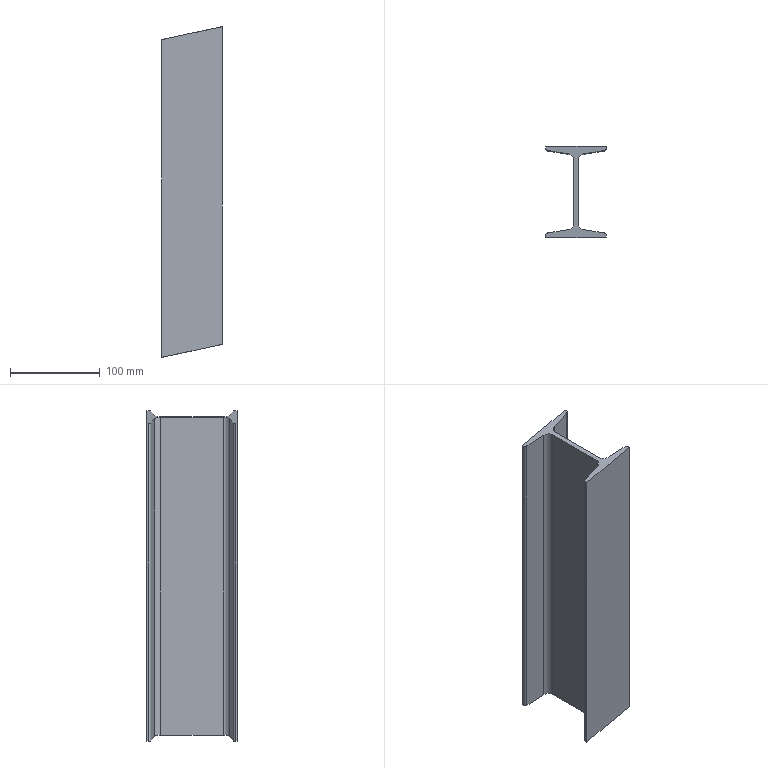Part | SolidWorks | features BaseBody 1 | 1 solid | 22 faces | box 67.6 x 101.6 x 369.5 mm | volume 493243 mm3 | plane 14 | cylinder 8 | commonest cylinder face diameters 5.6 x4 14.8 x4
STEP:
#1=CARTESIAN_POINT('',(50.959,42.223,361.667));
#2=VERTEX_POINT('',#1);
#3=CARTESIAN_POINT('',(50.959,112.103,361.667));
#4=VERTEX_POINT('',#3);
#5=CARTESIAN_POINT('',(50.959,42.223,361.667));
#6=DIRECTION('',(0.,1.,0.));
#7=VECTOR('',#6,1000.);
#8=LINE('',#5,#7);
#9=EDGE_CURVE('',#2,#4,#8,.T.);
#10=ORIENTED_EDGE('',*,*,#9,.T.);
#11=CARTESIAN_POINT('',(50.959,112.103,6.795));
#12=VERTEX_POINT('',#11);
#13=CARTESIAN_POINT('',(50.959,112.103,0.));
#14=DIRECTION('',(0.,0.,-1.));
#15=VECTOR('',#14,1000.);
#16=LINE('',#13,#15);
#17=EDGE_CURVE('',#4,#12,#16,.T.);
#18=ORIENTED_EDGE('',*,*,#17,.T.);
#19=CARTESIAN_POINT('',(50.959,42.223,6.795));
#20=VERTEX_POINT('',#19);
#21=CARTESIAN_POINT('',(50.959,42.223,6.795));
#22=DIRECTION('',(0.,-1.,0.));
#23=VECTOR('',#22,1000.);
#24=LINE('',#21,#23);
#25=EDGE_CURVE('',#12,#20,#24,.T.);
#26=ORIENTED_EDGE('',*,*,#25,.T.);
#27=CARTESIAN_POINT('',(50.959,42.223,0.));
#28=DIRECTION('',(0.,0.,1.));
#29=VECTOR('',#28,1000.);
#30=LINE('',#27,#29);
#31=EDGE_CURVE('',#20,#2,#30,.T.);
#32=ORIENTED_EDGE('',*,*,#31,.T.);
#33=EDGE_LOOP('',(#10,#18,#26,#32));
#34=FACE_OUTER_BOUND('',#33,.T.);
#35=CARTESIAN_POINT('',(50.959,42.223,0.));
#36=DIRECTION('',(-1.,0.,0.));
#37=DIRECTION('',(0.,0.,1.));
#38=AXIS2_PLACEMENT_3D('',#35,#36,#37);
#39=PLANE('',#38);
#40=ADVANCED_FACE('',(#34),#39,.T.);
#41=ORIENTED_EDGE('',*,*,#17,.F.);
#42=CARTESIAN_POINT('',(44.781,119.402,360.33));
#43=VERTEX_POINT('',#42);
#44=CARTESIAN_POINT('',(44.781,119.402,360.33));
#45=CARTESIAN_POINT('',(48.514,118.777,361.137));
#46=CARTESIAN_POINT('',(50.959,115.888,361.667));
#47=CARTESIAN_POINT('',(50.959,112.103,361.667));
#48=(BOUNDED_CURVE()B_SPLINE_CURVE(3,(#44,#45,#46,#47),.UNSPECIFIED.,.F.,.T.)B_SPLINE_CURVE_WITH_KNOTS((4,4),(4.878,6.283),.UNSPECIFIED.)CURVE()GEOMETRIC_REPRESENTATION_ITEM()RATIONAL_B_SPLINE_CURVE((1.,0.8422,0.8422,1.))REPRESENTATION_ITEM(''));
#49=EDGE_CURVE('',#43,#4,#48,.T.);
#50=ORIENTED_EDGE('',*,*,#49,.F.);
#51=CARTESIAN_POINT('',(44.781,119.402,5.458));
#52=VERTEX_POINT('',#51);
#53=CARTESIAN_POINT('',(44.781,119.402,0.));
#54=DIRECTION('',(0.,0.,1.));
#55=VECTOR('',#54,1000.);
#56=LINE('',#53,#55);
#57=EDGE_CURVE('',#52,#43,#56,.T.);
#58=ORIENTED_EDGE('',*,*,#57,.F.);
#59=CARTESIAN_POINT('',(50.959,112.103,6.795));
#60=CARTESIAN_POINT('',(50.959,115.888,6.795));
#61=CARTESIAN_POINT('',(48.514,118.777,6.265));
#62=CARTESIAN_POINT('',(44.781,119.402,5.458));
#63=(BOUNDED_CURVE()B_SPLINE_CURVE(3,(#59,#60,#61,#62),.UNSPECIFIED.,.F.,.T.)B_SPLINE_CURVE_WITH_KNOTS((4,4),(0.,1.405),.UNSPECIFIED.)CURVE()GEOMETRIC_REPRESENTATION_ITEM()RATIONAL_B_SPLINE_CURVE((1.,0.8422,0.8422,1.))REPRESENTATION_ITEM(''));
#64=EDGE_CURVE('',#12,#52,#63,.T.);
#65=ORIENTED_EDGE('',*,*,#64,.F.);
#66=EDGE_LOOP('',(#41,#50,#58,#65));
#67=FACE_OUTER_BOUND('',#66,.T.);
#68=CARTESIAN_POINT('',(43.559,112.103,0.));
#69=DIRECTION('',(0.,0.,1.));
#70=DIRECTION('',(1.,0.,0.));
#71=AXIS2_PLACEMENT_3D('',#68,#69,#70);
#72=CYLINDRICAL_SURFACE('',#71,7.4);
#73=ADVANCED_FACE('',(#67),#72,.F.);
#74=CARTESIAN_POINT('',(87.159,26.363,369.5));
#75=VERTEX_POINT('',#74);
#76=CARTESIAN_POINT('',(19.559,26.363,354.872));
#77=VERTEX_POINT('',#76);
#78=CARTESIAN_POINT('',(4.183,26.363,351.545));
#79=DIRECTION('',(-0.9774,0.,-0.2115));
#80=VECTOR('',#79,1000.);
#81=LINE('',#78,#80);
#82=EDGE_CURVE('',#75,#77,#81,.T.);
#83=ORIENTED_EDGE('',*,*,#82,.F.);
#84=CARTESIAN_POINT('',(87.159,28.334,369.5));
#85=VERTEX_POINT('',#84);
#86=CARTESIAN_POINT('',(87.159,26.363,369.5));
#87=DIRECTION('',(0.,-1.,0.));
#88=VECTOR('',#87,1000.);
#89=LINE('',#86,#88);
#90=EDGE_CURVE('',#85,#75,#89,.T.);
#91=ORIENTED_EDGE('',*,*,#90,.F.);
#92=CARTESIAN_POINT('',(84.821,31.095,368.994));
#93=VERTEX_POINT('',#92);
#94=CARTESIAN_POINT('',(84.821,31.095,368.994));
#95=CARTESIAN_POINT('',(86.234,30.859,369.3));
#96=CARTESIAN_POINT('',(87.159,29.766,369.5));
#97=CARTESIAN_POINT('',(87.159,28.334,369.5));
#98=(BOUNDED_CURVE()B_SPLINE_CURVE(3,(#94,#95,#96,#97),.UNSPECIFIED.,.F.,.T.)B_SPLINE_CURVE_WITH_KNOTS((4,4),(4.878,6.283),.UNSPECIFIED.)CURVE()GEOMETRIC_REPRESENTATION_ITEM()RATIONAL_B_SPLINE_CURVE((1.,0.8422,0.8422,1.))REPRESENTATION_ITEM(''));
#99=EDGE_CURVE('',#93,#85,#98,.T.);
#100=ORIENTED_EDGE('',*,*,#99,.F.);
#101=CARTESIAN_POINT('',(61.938,34.925,364.042));
#102=VERTEX_POINT('',#101);
#103=CARTESIAN_POINT('',(61.938,34.925,364.042));
#104=DIRECTION('',(0.9646,-0.1614,0.2087));
#105=VECTOR('',#104,1000.);
#106=LINE('',#103,#105);
#107=EDGE_CURVE('',#102,#93,#106,.T.);
#108=ORIENTED_EDGE('',*,*,#107,.F.);
#109=CARTESIAN_POINT('',(55.759,42.223,362.705));
#110=VERTEX_POINT('',#109);
#111=CARTESIAN_POINT('',(55.759,42.223,362.705));
#112=CARTESIAN_POINT('',(55.759,38.438,362.705));
#113=CARTESIAN_POINT('',(58.205,35.55,363.235));
#114=CARTESIAN_POINT('',(61.938,34.925,364.042));
#115=(BOUNDED_CURVE()B_SPLINE_CURVE(3,(#111,#112,#113,#114),.UNSPECIFIED.,.F.,.F.)B_SPLINE_CURVE_WITH_KNOTS((4,4),(3.142,4.547),.UNSPECIFIED.)CURVE()GEOMETRIC_REPRESENTATION_ITEM()RATIONAL_B_SPLINE_CURVE((1.,0.8422,0.8422,1.))REPRESENTATION_ITEM(''));
#116=EDGE_CURVE('',#110,#102,#115,.T.);
#117=ORIENTED_EDGE('',*,*,#116,.F.);
#118=CARTESIAN_POINT('',(55.759,112.103,362.705));
#119=VERTEX_POINT('',#118);
#120=CARTESIAN_POINT('',(55.759,26.363,362.705));
#121=DIRECTION('',(0.,-1.,0.));
#122=VECTOR('',#121,1000.);
#123=LINE('',#120,#122);
#124=EDGE_CURVE('',#119,#110,#123,.T.);
#125=ORIENTED_EDGE('',*,*,#124,.F.);
#126=CARTESIAN_POINT('',(61.938,119.402,364.042));
#127=VERTEX_POINT('',#126);
#128=CARTESIAN_POINT('',(61.938,119.402,364.042));
#129=CARTESIAN_POINT('',(58.205,118.777,363.235));
#130=CARTESIAN_POINT('',(55.759,115.888,362.705));
#131=CARTESIAN_POINT('',(55.759,112.103,362.705));
#132=(BOUNDED_CURVE()B_SPLINE_CURVE(3,(#128,#129,#130,#131),.UNSPECIFIED.,.F.,.T.)B_SPLINE_CURVE_WITH_KNOTS((4,4),(1.737,3.142),.UNSPECIFIED.)CURVE()GEOMETRIC_REPRESENTATION_ITEM()RATIONAL_B_SPLINE_CURVE((1.,0.8422,0.8422,1.))REPRESENTATION_ITEM(''));
#133=EDGE_CURVE('',#127,#119,#132,.T.);
#134=ORIENTED_EDGE('',*,*,#133,.F.);
#135=CARTESIAN_POINT('',(84.821,123.231,368.994));
#136=VERTEX_POINT('',#135);
#137=CARTESIAN_POINT('',(84.821,123.231,368.994));
#138=DIRECTION('',(-0.9646,-0.1614,-0.2087));
#139=VECTOR('',#138,1000.);
#140=LINE('',#137,#139);
#141=EDGE_CURVE('',#136,#127,#140,.T.);
#142=ORIENTED_EDGE('',*,*,#141,.F.);
#143=CARTESIAN_POINT('',(87.159,125.993,369.5));
#144=VERTEX_POINT('',#143);
#145=CARTESIAN_POINT('',(87.159,125.993,369.5));
#146=CARTESIAN_POINT('',(87.159,124.561,369.5));
#147=CARTESIAN_POINT('',(86.234,123.468,369.3));
#148=CARTESIAN_POINT('',(84.821,123.231,368.994));
#149=(BOUNDED_CURVE()B_SPLINE_CURVE(3,(#145,#146,#147,#148),.UNSPECIFIED.,.F.,.F.)B_SPLINE_CURVE_WITH_KNOTS((4,4),(0.,1.405),.UNSPECIFIED.)CURVE()GEOMETRIC_REPRESENTATION_ITEM()RATIONAL_B_SPLINE_CURVE((1.,0.8422,0.8422,1.))REPRESENTATION_ITEM(''));
#150=EDGE_CURVE('',#144,#136,#149,.T.);
#151=ORIENTED_EDGE('',*,*,#150,.F.);
#152=CARTESIAN_POINT('',(87.159,127.963,369.5));
#153=VERTEX_POINT('',#152);
#154=CARTESIAN_POINT('',(87.159,26.363,369.5));
#155=DIRECTION('',(0.,-1.,0.));
#156=VECTOR('',#155,1000.);
#157=LINE('',#154,#156);
#158=EDGE_CURVE('',#153,#144,#157,.T.);
#159=ORIENTED_EDGE('',*,*,#158,.F.);
#160=CARTESIAN_POINT('',(19.559,127.963,354.872));
#161=VERTEX_POINT('',#160);
#162=CARTESIAN_POINT('',(4.183,127.963,351.545));
#163=DIRECTION('',(0.9774,0.,0.2115));
#164=VECTOR('',#163,1000.);
#165=LINE('',#162,#164);
#166=EDGE_CURVE('',#161,#153,#165,.T.);
#167=ORIENTED_EDGE('',*,*,#166,.F.);
#168=CARTESIAN_POINT('',(19.559,125.993,354.872));
#169=VERTEX_POINT('',#168);
#170=CARTESIAN_POINT('',(19.559,26.363,354.872));
#171=DIRECTION('',(0.,1.,0.));
#172=VECTOR('',#171,1000.);
#173=LINE('',#170,#172);
#174=EDGE_CURVE('',#169,#161,#173,.T.);
#175=ORIENTED_EDGE('',*,*,#174,.F.);
#176=CARTESIAN_POINT('',(21.897,123.231,355.378));
#177=VERTEX_POINT('',#176);
#178=CARTESIAN_POINT('',(21.897,123.231,355.378));
#179=CARTESIAN_POINT('',(20.485,123.468,355.072));
#180=CARTESIAN_POINT('',(19.559,124.561,354.872));
#181=CARTESIAN_POINT('',(19.559,125.993,354.872));
#182=(BOUNDED_CURVE()B_SPLINE_CURVE(3,(#178,#179,#180,#181),.UNSPECIFIED.,.F.,.T.)B_SPLINE_CURVE_WITH_KNOTS((4,4),(1.737,3.142),.UNSPECIFIED.)CURVE()GEOMETRIC_REPRESENTATION_ITEM()RATIONAL_B_SPLINE_CURVE((1.,0.8422,0.8422,1.))REPRESENTATION_ITEM(''));
#183=EDGE_CURVE('',#177,#169,#182,.T.);
#184=ORIENTED_EDGE('',*,*,#183,.F.);
#185=CARTESIAN_POINT('',(44.781,119.402,360.33));
#186=DIRECTION('',(-0.9646,0.1614,-0.2087));
#187=VECTOR('',#186,1000.);
#188=LINE('',#185,#187);
#189=EDGE_CURVE('',#43,#177,#188,.T.);
#190=ORIENTED_EDGE('',*,*,#189,.F.);
#191=ORIENTED_EDGE('',*,*,#49,.T.);
#192=ORIENTED_EDGE('',*,*,#9,.F.);
#193=CARTESIAN_POINT('',(44.781,34.925,360.33));
#194=VERTEX_POINT('',#193);
#195=CARTESIAN_POINT('',(44.781,34.925,360.33));
#196=CARTESIAN_POINT('',(48.514,35.55,361.137));
#197=CARTESIAN_POINT('',(50.959,38.438,361.667));
#198=CARTESIAN_POINT('',(50.959,42.223,361.667));
#199=(BOUNDED_CURVE()B_SPLINE_CURVE(3,(#195,#196,#197,#198),.UNSPECIFIED.,.F.,.T.)B_SPLINE_CURVE_WITH_KNOTS((4,4),(4.878,6.283),.UNSPECIFIED.)CURVE()GEOMETRIC_REPRESENTATION_ITEM()RATIONAL_B_SPLINE_CURVE((1.,0.8422,0.8422,1.))REPRESENTATION_ITEM(''));
#200=EDGE_CURVE('',#194,#2,#199,.T.);
#201=ORIENTED_EDGE('',*,*,#200,.F.);
#202=CARTESIAN_POINT('',(21.897,31.095,355.378));
#203=VERTEX_POINT('',#202);
#204=CARTESIAN_POINT('',(21.897,31.095,355.378));
#205=DIRECTION('',(0.9646,0.1614,0.2087));
#206=VECTOR('',#205,1000.);
#207=LINE('',#204,#206);
#208=EDGE_CURVE('',#203,#194,#207,.T.);
#209=ORIENTED_EDGE('',*,*,#208,.F.);
#210=CARTESIAN_POINT('',(19.559,28.334,354.872));
#211=VERTEX_POINT('',#210);
#212=CARTESIAN_POINT('',(19.559,28.334,354.872));
#213=CARTESIAN_POINT('',(19.559,29.766,354.872));
#214=CARTESIAN_POINT('',(20.485,30.859,355.072));
#215=CARTESIAN_POINT('',(21.897,31.095,355.378));
#216=(BOUNDED_CURVE()B_SPLINE_CURVE(3,(#212,#213,#214,#215),.UNSPECIFIED.,.F.,.T.)B_SPLINE_CURVE_WITH_KNOTS((4,4),(3.142,4.547),.UNSPECIFIED.)CURVE()GEOMETRIC_REPRESENTATION_ITEM()RATIONAL_B_SPLINE_CURVE((1.,0.8422,0.8422,1.))REPRESENTATION_ITEM(''));
#217=EDGE_CURVE('',#211,#203,#216,.T.);
#218=ORIENTED_EDGE('',*,*,#217,.F.);
#219=CARTESIAN_POINT('',(19.559,26.363,354.872));
#220=DIRECTION('',(0.,1.,0.));
#221=VECTOR('',#220,1000.);
#222=LINE('',#219,#221);
#223=EDGE_CURVE('',#77,#211,#222,.T.);
#224=ORIENTED_EDGE('',*,*,#223,.F.);
#225=EDGE_LOOP('',(#83,#91,#100,#108,#117,#125,#134,#142,#151,#159,#167,#175,#184,#190,#191,#192,#201,#209,#218,#224));
#226=FACE_OUTER_BOUND('',#225,.T.);
#227=CARTESIAN_POINT('',(4.183,26.363,351.545));
#228=DIRECTION('',(0.2115,0.,-0.9774));
#229=DIRECTION('',(-0.9774,0.,-0.2115));
#230=AXIS2_PLACEMENT_3D('',#227,#228,#229);
#231=PLANE('',#230);
#232=ADVANCED_FACE('',(#226),#231,.F.);
#233=CARTESIAN_POINT('',(44.781,34.925,5.458));
#234=VERTEX_POINT('',#233);
#235=CARTESIAN_POINT('',(44.781,34.925,0.));
#236=DIRECTION('',(0.,0.,-1.));
#237=VECTOR('',#236,1000.);
#238=LINE('',#235,#237);
#239=EDGE_CURVE('',#194,#234,#238,.T.);
#240=ORIENTED_EDGE('',*,*,#239,.F.);
#241=ORIENTED_EDGE('',*,*,#200,.T.);
#242=ORIENTED_EDGE('',*,*,#31,.F.);
#243=CARTESIAN_POINT('',(44.781,34.925,5.458));
#244=CARTESIAN_POINT('',(48.514,35.55,6.265));
#245=CARTESIAN_POINT('',(50.959,38.438,6.795));
#246=CARTESIAN_POINT('',(50.959,42.223,6.795));
#247=(BOUNDED_CURVE()B_SPLINE_CURVE(3,(#243,#244,#245,#246),.UNSPECIFIED.,.F.,.T.)B_SPLINE_CURVE_WITH_KNOTS((4,4),(4.878,6.283),.UNSPECIFIED.)CURVE()GEOMETRIC_REPRESENTATION_ITEM()RATIONAL_B_SPLINE_CURVE((1.,0.8422,0.8422,1.))REPRESENTATION_ITEM(''));
#248=EDGE_CURVE('',#234,#20,#247,.T.);
#249=ORIENTED_EDGE('',*,*,#248,.F.);
#250=EDGE_LOOP('',(#240,#241,#242,#249));
#251=FACE_OUTER_BOUND('',#250,.T.);
#252=CARTESIAN_POINT('',(43.559,42.223,0.));
#253=DIRECTION('',(0.,0.,1.));
#254=DIRECTION('',(1.,0.,0.));
#255=AXIS2_PLACEMENT_3D('',#252,#253,#254);
#256=CYLINDRICAL_SURFACE('',#255,7.4);
#257=ADVANCED_FACE('',(#251),#256,.F.);
#258=CARTESIAN_POINT('',(19.559,26.363,0.));
#259=VERTEX_POINT('',#258);
#260=CARTESIAN_POINT('',(87.159,26.363,14.628));
#261=VERTEX_POINT('',#260);
#262=CARTESIAN_POINT('',(101.44,26.363,17.718));
#263=DIRECTION('',(0.9774,0.,0.2115));
#264=VECTOR('',#263,1000.);
#265=LINE('',#262,#264);
#266=EDGE_CURVE('',#259,#261,#265,.T.);
#267=ORIENTED_EDGE('',*,*,#266,.F.);
#268=CARTESIAN_POINT('',(19.559,28.334,0.));
#269=VERTEX_POINT('',#268);
#270=CARTESIAN_POINT('',(19.559,26.363,0.));
#271=DIRECTION('',(0.,-1.,0.));
#272=VECTOR('',#271,1000.);
#273=LINE('',#270,#272);
#274=EDGE_CURVE('',#269,#259,#273,.T.);
#275=ORIENTED_EDGE('',*,*,#274,.F.);
#276=CARTESIAN_POINT('',(21.897,31.095,0.5059));
#277=VERTEX_POINT('',#276);
#278=CARTESIAN_POINT('',(21.897,31.095,0.5059));
#279=CARTESIAN_POINT('',(20.485,30.859,0.2002));
#280=CARTESIAN_POINT('',(19.559,29.766,0.));
#281=CARTESIAN_POINT('',(19.559,28.334,0.));
#282=(BOUNDED_CURVE()B_SPLINE_CURVE(3,(#278,#279,#280,#281),.UNSPECIFIED.,.F.,.T.)B_SPLINE_CURVE_WITH_KNOTS((4,4),(1.737,3.142),.UNSPECIFIED.)CURVE()GEOMETRIC_REPRESENTATION_ITEM()RATIONAL_B_SPLINE_CURVE((1.,0.8422,0.8422,1.))REPRESENTATION_ITEM(''));
#283=EDGE_CURVE('',#277,#269,#282,.T.);
#284=ORIENTED_EDGE('',*,*,#283,.F.);
#285=CARTESIAN_POINT('',(44.781,34.925,5.458));
#286=DIRECTION('',(-0.9646,-0.1614,-0.2087));
#287=VECTOR('',#286,1000.);
#288=LINE('',#285,#287);
#289=EDGE_CURVE('',#234,#277,#288,.T.);
#290=ORIENTED_EDGE('',*,*,#289,.F.);
#291=ORIENTED_EDGE('',*,*,#248,.T.);
#292=ORIENTED_EDGE('',*,*,#25,.F.);
#293=ORIENTED_EDGE('',*,*,#64,.T.);
#294=CARTESIAN_POINT('',(21.897,123.231,0.5059));
#295=VERTEX_POINT('',#294);
#296=CARTESIAN_POINT('',(21.897,123.231,0.5059));
#297=DIRECTION('',(0.9646,-0.1614,0.2087));
#298=VECTOR('',#297,1000.);
#299=LINE('',#296,#298);
#300=EDGE_CURVE('',#295,#52,#299,.T.);
#301=ORIENTED_EDGE('',*,*,#300,.F.);
#302=CARTESIAN_POINT('',(19.559,125.993,0.));
#303=VERTEX_POINT('',#302);
#304=CARTESIAN_POINT('',(19.559,125.993,0.));
#305=CARTESIAN_POINT('',(19.559,124.561,0.));
#306=CARTESIAN_POINT('',(20.485,123.468,0.2002));
#307=CARTESIAN_POINT('',(21.897,123.231,0.5059));
#308=(BOUNDED_CURVE()B_SPLINE_CURVE(3,(#304,#305,#306,#307),.UNSPECIFIED.,.F.,.T.)B_SPLINE_CURVE_WITH_KNOTS((4,4),(3.142,4.547),.UNSPECIFIED.)CURVE()GEOMETRIC_REPRESENTATION_ITEM()RATIONAL_B_SPLINE_CURVE((1.,0.8422,0.8422,1.))REPRESENTATION_ITEM(''));
#309=EDGE_CURVE('',#303,#295,#308,.T.);
#310=ORIENTED_EDGE('',*,*,#309,.F.);
#311=CARTESIAN_POINT('',(19.559,127.963,0.));
#312=VERTEX_POINT('',#311);
#313=CARTESIAN_POINT('',(19.559,26.363,0.));
#314=DIRECTION('',(0.,-1.,0.));
#315=VECTOR('',#314,1000.);
#316=LINE('',#313,#315);
#317=EDGE_CURVE('',#312,#303,#316,.T.);
#318=ORIENTED_EDGE('',*,*,#317,.F.);
#319=CARTESIAN_POINT('',(87.159,127.963,14.628));
#320=VERTEX_POINT('',#319);
#321=CARTESIAN_POINT('',(101.44,127.963,17.718));
#322=DIRECTION('',(-0.9774,0.,-0.2115));
#323=VECTOR('',#322,1000.);
#324=LINE('',#321,#323);
#325=EDGE_CURVE('',#320,#312,#324,.T.);
#326=ORIENTED_EDGE('',*,*,#325,.F.);
#327=CARTESIAN_POINT('',(87.159,125.993,14.628));
#328=VERTEX_POINT('',#327);
#329=CARTESIAN_POINT('',(87.159,26.363,14.628));
#330=DIRECTION('',(0.,1.,0.));
#331=VECTOR('',#330,1000.);
#332=LINE('',#329,#331);
#333=EDGE_CURVE('',#328,#320,#332,.T.);
#334=ORIENTED_EDGE('',*,*,#333,.F.);
#335=CARTESIAN_POINT('',(84.821,123.231,14.122));
#336=VERTEX_POINT('',#335);
#337=CARTESIAN_POINT('',(84.821,123.231,14.122));
#338=CARTESIAN_POINT('',(86.234,123.468,14.428));
#339=CARTESIAN_POINT('',(87.159,124.561,14.628));
#340=CARTESIAN_POINT('',(87.159,125.993,14.628));
#341=(BOUNDED_CURVE()B_SPLINE_CURVE(3,(#337,#338,#339,#340),.UNSPECIFIED.,.F.,.T.)B_SPLINE_CURVE_WITH_KNOTS((4,4),(4.878,6.283),.UNSPECIFIED.)CURVE()GEOMETRIC_REPRESENTATION_ITEM()RATIONAL_B_SPLINE_CURVE((1.,0.8422,0.8422,1.))REPRESENTATION_ITEM(''));
#342=EDGE_CURVE('',#336,#328,#341,.T.);
#343=ORIENTED_EDGE('',*,*,#342,.F.);
#344=CARTESIAN_POINT('',(61.938,119.402,9.17));
#345=VERTEX_POINT('',#344);
#346=CARTESIAN_POINT('',(61.938,119.402,9.17));
#347=DIRECTION('',(0.9646,0.1614,0.2087));
#348=VECTOR('',#347,1000.);
#349=LINE('',#346,#348);
#350=EDGE_CURVE('',#345,#336,#349,.T.);
#351=ORIENTED_EDGE('',*,*,#350,.F.);
#352=CARTESIAN_POINT('',(55.759,112.103,7.833));
#353=VERTEX_POINT('',#352);
#354=CARTESIAN_POINT('',(55.759,112.103,7.833));
#355=CARTESIAN_POINT('',(55.759,115.888,7.833));
#356=CARTESIAN_POINT('',(58.205,118.777,8.363));
#357=CARTESIAN_POINT('',(61.938,119.402,9.17));
#358=(BOUNDED_CURVE()B_SPLINE_CURVE(3,(#354,#355,#356,#357),.UNSPECIFIED.,.F.,.T.)B_SPLINE_CURVE_WITH_KNOTS((4,4),(3.142,4.547),.UNSPECIFIED.)CURVE()GEOMETRIC_REPRESENTATION_ITEM()RATIONAL_B_SPLINE_CURVE((1.,0.8422,0.8422,1.))REPRESENTATION_ITEM(''));
#359=EDGE_CURVE('',#353,#345,#358,.T.);
#360=ORIENTED_EDGE('',*,*,#359,.F.);
#361=CARTESIAN_POINT('',(55.759,42.223,7.833));
#362=VERTEX_POINT('',#361);
#363=CARTESIAN_POINT('',(55.759,26.363,7.833));
#364=DIRECTION('',(0.,1.,0.));
#365=VECTOR('',#364,1000.);
#366=LINE('',#363,#365);
#367=EDGE_CURVE('',#362,#353,#366,.T.);
#368=ORIENTED_EDGE('',*,*,#367,.F.);
#369=CARTESIAN_POINT('',(61.938,34.925,9.17));
#370=VERTEX_POINT('',#369);
#371=CARTESIAN_POINT('',(61.938,34.925,9.17));
#372=CARTESIAN_POINT('',(58.205,35.55,8.363));
#373=CARTESIAN_POINT('',(55.759,38.438,7.833));
#374=CARTESIAN_POINT('',(55.759,42.223,7.833));
#375=(BOUNDED_CURVE()B_SPLINE_CURVE(3,(#371,#372,#373,#374),.UNSPECIFIED.,.F.,.F.)B_SPLINE_CURVE_WITH_KNOTS((4,4),(1.737,3.142),.UNSPECIFIED.)CURVE()GEOMETRIC_REPRESENTATION_ITEM()RATIONAL_B_SPLINE_CURVE((1.,0.8422,0.8422,1.))REPRESENTATION_ITEM(''));
#376=EDGE_CURVE('',#370,#362,#375,.T.);
#377=ORIENTED_EDGE('',*,*,#376,.F.);
#378=CARTESIAN_POINT('',(84.821,31.095,14.122));
#379=VERTEX_POINT('',#378);
#380=CARTESIAN_POINT('',(84.821,31.095,14.122));
#381=DIRECTION('',(-0.9646,0.1614,-0.2087));
#382=VECTOR('',#381,1000.);
#383=LINE('',#380,#382);
#384=EDGE_CURVE('',#379,#370,#383,.T.);
#385=ORIENTED_EDGE('',*,*,#384,.F.);
#386=CARTESIAN_POINT('',(87.159,28.334,14.628));
#387=VERTEX_POINT('',#386);
#388=CARTESIAN_POINT('',(87.159,28.334,14.628));
#389=CARTESIAN_POINT('',(87.159,29.766,14.628));
#390=CARTESIAN_POINT('',(86.234,30.859,14.428));
#391=CARTESIAN_POINT('',(84.821,31.095,14.122));
#392=(BOUNDED_CURVE()B_SPLINE_CURVE(3,(#388,#389,#390,#391),.UNSPECIFIED.,.F.,.T.)B_SPLINE_CURVE_WITH_KNOTS((4,4),(0.,1.405),.UNSPECIFIED.)CURVE()GEOMETRIC_REPRESENTATION_ITEM()RATIONAL_B_SPLINE_CURVE((1.,0.8422,0.8422,1.))REPRESENTATION_ITEM(''));
#393=EDGE_CURVE('',#387,#379,#392,.T.);
#394=ORIENTED_EDGE('',*,*,#393,.F.);
#395=CARTESIAN_POINT('',(87.159,26.363,14.628));
#396=DIRECTION('',(0.,1.,0.));
#397=VECTOR('',#396,1000.);
#398=LINE('',#395,#397);
#399=EDGE_CURVE('',#261,#387,#398,.T.);
#400=ORIENTED_EDGE('',*,*,#399,.F.);
#401=EDGE_LOOP('',(#267,#275,#284,#290,#291,#292,#293,#301,#310,#318,#326,#334,#343,#351,#360,#368,#377,#385,#394,#400));
#402=FACE_OUTER_BOUND('',#401,.T.);
#403=CARTESIAN_POINT('',(101.44,26.363,17.718));
#404=DIRECTION('',(-0.2115,0.,0.9774));
#405=DIRECTION('',(0.9774,0.,0.2115));
#406=AXIS2_PLACEMENT_3D('',#403,#404,#405);
#407=PLANE('',#406);
#408=ADVANCED_FACE('',(#402),#407,.F.);
#409=ORIENTED_EDGE('',*,*,#189,.T.);
#410=CARTESIAN_POINT('',(21.897,123.231,0.));
#411=DIRECTION('',(0.,0.,-1.));
#412=VECTOR('',#411,1000.);
#413=LINE('',#410,#412);
#414=EDGE_CURVE('',#177,#295,#413,.T.);
#415=ORIENTED_EDGE('',*,*,#414,.T.);
#416=ORIENTED_EDGE('',*,*,#300,.T.);
#417=ORIENTED_EDGE('',*,*,#57,.T.);
#418=EDGE_LOOP('',(#409,#415,#416,#417));
#419=FACE_OUTER_BOUND('',#418,.T.);
#420=CARTESIAN_POINT('',(44.781,119.402,0.));
#421=DIRECTION('',(-0.165,-0.9863,0.));
#422=DIRECTION('',(0.9863,-0.165,0.));
#423=AXIS2_PLACEMENT_3D('',#420,#421,#422);
#424=PLANE('',#423);
#425=ADVANCED_FACE('',(#419),#424,.T.);
#426=ORIENTED_EDGE('',*,*,#274,.T.);
#427=CARTESIAN_POINT('',(19.559,26.363,0.));
#428=DIRECTION('',(0.,0.,1.));
#429=VECTOR('',#428,1000.);
#430=LINE('',#427,#429);
#431=EDGE_CURVE('',#259,#77,#430,.T.);
#432=ORIENTED_EDGE('',*,*,#431,.T.);
#433=ORIENTED_EDGE('',*,*,#223,.T.);
#434=CARTESIAN_POINT('',(19.559,28.334,0.));
#435=DIRECTION('',(0.,0.,-1.));
#436=VECTOR('',#435,1000.);
#437=LINE('',#434,#436);
#438=EDGE_CURVE('',#211,#269,#437,.T.);
#439=ORIENTED_EDGE('',*,*,#438,.T.);
#440=EDGE_LOOP('',(#426,#432,#433,#439));
#441=FACE_OUTER_BOUND('',#440,.T.);
#442=CARTESIAN_POINT('',(19.559,26.363,0.));
#443=DIRECTION('',(-1.,0.,0.));
#444=DIRECTION('',(0.,-1.,0.));
#445=AXIS2_PLACEMENT_3D('',#442,#443,#444);
#446=PLANE('',#445);
#447=ADVANCED_FACE('',(#441),#446,.T.);
#448=ORIENTED_EDGE('',*,*,#82,.T.);
#449=ORIENTED_EDGE('',*,*,#431,.F.);
#450=ORIENTED_EDGE('',*,*,#266,.T.);
#451=CARTESIAN_POINT('',(87.159,26.363,0.));
#452=DIRECTION('',(0.,0.,1.));
#453=VECTOR('',#452,1000.);
#454=LINE('',#451,#453);
#455=EDGE_CURVE('',#261,#75,#454,.T.);
#456=ORIENTED_EDGE('',*,*,#455,.T.);
#457=EDGE_LOOP('',(#448,#449,#450,#456));
#458=FACE_OUTER_BOUND('',#457,.T.);
#459=CARTESIAN_POINT('',(87.159,26.363,0.));
#460=DIRECTION('',(0.,-1.,0.));
#461=DIRECTION('',(0.,0.,-1.));
#462=AXIS2_PLACEMENT_3D('',#459,#460,#461);
#463=PLANE('',#462);
#464=ADVANCED_FACE('',(#458),#463,.T.);
#465=ORIENTED_EDGE('',*,*,#90,.T.);
#466=ORIENTED_EDGE('',*,*,#455,.F.);
#467=ORIENTED_EDGE('',*,*,#399,.T.);
#468=CARTESIAN_POINT('',(87.159,28.334,0.));
#469=DIRECTION('',(0.,0.,1.));
#470=VECTOR('',#469,1000.);
#471=LINE('',#468,#470);
#472=EDGE_CURVE('',#387,#85,#471,.T.);
#473=ORIENTED_EDGE('',*,*,#472,.T.);
#474=EDGE_LOOP('',(#465,#466,#467,#473));
#475=FACE_OUTER_BOUND('',#474,.T.);
#476=CARTESIAN_POINT('',(87.159,28.334,0.));
#477=DIRECTION('',(1.,0.,0.));
#478=DIRECTION('',(0.,1.,0.));
#479=AXIS2_PLACEMENT_3D('',#476,#477,#478);
#480=PLANE('',#479);
#481=ADVANCED_FACE('',(#475),#480,.T.);
#482=ORIENTED_EDGE('',*,*,#99,.T.);
#483=ORIENTED_EDGE('',*,*,#472,.F.);
#484=ORIENTED_EDGE('',*,*,#393,.T.);
#485=CARTESIAN_POINT('',(84.821,31.095,0.));
#486=DIRECTION('',(0.,0.,1.));
#487=VECTOR('',#486,1000.);
#488=LINE('',#485,#487);
#489=EDGE_CURVE('',#379,#93,#488,.T.);
#490=ORIENTED_EDGE('',*,*,#489,.T.);
#491=EDGE_LOOP('',(#482,#483,#484,#490));
#492=FACE_OUTER_BOUND('',#491,.T.);
#493=CARTESIAN_POINT('',(84.359,28.334,0.));
#494=DIRECTION('',(0.,0.,1.));
#495=DIRECTION('',(1.,0.,0.));
#496=AXIS2_PLACEMENT_3D('',#493,#494,#495);
#497=CYLINDRICAL_SURFACE('',#496,2.8);
#498=ADVANCED_FACE('',(#492),#497,.T.);
#499=ORIENTED_EDGE('',*,*,#107,.T.);
#500=ORIENTED_EDGE('',*,*,#489,.F.);
#501=ORIENTED_EDGE('',*,*,#384,.T.);
#502=CARTESIAN_POINT('',(61.938,34.925,0.));
#503=DIRECTION('',(0.,0.,1.));
#504=VECTOR('',#503,1000.);
#505=LINE('',#502,#504);
#506=EDGE_CURVE('',#370,#102,#505,.T.);
#507=ORIENTED_EDGE('',*,*,#506,.T.);
#508=EDGE_LOOP('',(#499,#500,#501,#507));
#509=FACE_OUTER_BOUND('',#508,.T.);
#510=CARTESIAN_POINT('',(61.938,34.925,0.));
#511=DIRECTION('',(0.165,0.9863,0.));
#512=DIRECTION('',(-0.9863,0.165,0.));
#513=AXIS2_PLACEMENT_3D('',#510,#511,#512);
#514=PLANE('',#513);
#515=ADVANCED_FACE('',(#509),#514,.T.);
#516=CARTESIAN_POINT('',(55.759,42.223,0.));
#517=DIRECTION('',(0.,0.,-1.));
#518=VECTOR('',#517,1000.);
#519=LINE('',#516,#518);
#520=EDGE_CURVE('',#110,#362,#519,.T.);
#521=ORIENTED_EDGE('',*,*,#520,.F.);
#522=ORIENTED_EDGE('',*,*,#116,.T.);
#523=ORIENTED_EDGE('',*,*,#506,.F.);
#524=ORIENTED_EDGE('',*,*,#376,.T.);
#525=EDGE_LOOP('',(#521,#522,#523,#524));
#526=FACE_OUTER_BOUND('',#525,.T.);
#527=CARTESIAN_POINT('',(63.159,42.223,0.));
#528=DIRECTION('',(0.,0.,1.));
#529=DIRECTION('',(1.,0.,0.));
#530=AXIS2_PLACEMENT_3D('',#527,#528,#529);
#531=CYLINDRICAL_SURFACE('',#530,7.4);
#532=ADVANCED_FACE('',(#526),#531,.F.);
#533=ORIENTED_EDGE('',*,*,#124,.T.);
#534=ORIENTED_EDGE('',*,*,#520,.T.);
#535=ORIENTED_EDGE('',*,*,#367,.T.);
#536=CARTESIAN_POINT('',(55.759,112.103,0.));
#537=DIRECTION('',(0.,0.,1.));
#538=VECTOR('',#537,1000.);
#539=LINE('',#536,#538);
#540=EDGE_CURVE('',#353,#119,#539,.T.);
#541=ORIENTED_EDGE('',*,*,#540,.T.);
#542=EDGE_LOOP('',(#533,#534,#535,#541));
#543=FACE_OUTER_BOUND('',#542,.T.);
#544=CARTESIAN_POINT('',(55.759,112.103,0.));
#545=DIRECTION('',(1.,0.,0.));
#546=DIRECTION('',(0.,0.,-1.));
#547=AXIS2_PLACEMENT_3D('',#544,#545,#546);
#548=PLANE('',#547);
#549=ADVANCED_FACE('',(#543),#548,.T.);
#550=CARTESIAN_POINT('',(61.938,119.402,0.));
#551=DIRECTION('',(0.,0.,-1.));
#552=VECTOR('',#551,1000.);
#553=LINE('',#550,#552);
#554=EDGE_CURVE('',#127,#345,#553,.T.);
#555=ORIENTED_EDGE('',*,*,#554,.F.);
#556=ORIENTED_EDGE('',*,*,#133,.T.);
#557=ORIENTED_EDGE('',*,*,#540,.F.);
#558=ORIENTED_EDGE('',*,*,#359,.T.);
#559=EDGE_LOOP('',(#555,#556,#557,#558));
#560=FACE_OUTER_BOUND('',#559,.T.);
#561=CARTESIAN_POINT('',(63.159,112.103,0.));
#562=DIRECTION('',(0.,0.,1.));
#563=DIRECTION('',(1.,0.,0.));
#564=AXIS2_PLACEMENT_3D('',#561,#562,#563);
#565=CYLINDRICAL_SURFACE('',#564,7.4);
#566=ADVANCED_FACE('',(#560),#565,.F.);
#567=ORIENTED_EDGE('',*,*,#141,.T.);
#568=ORIENTED_EDGE('',*,*,#554,.T.);
#569=ORIENTED_EDGE('',*,*,#350,.T.);
#570=CARTESIAN_POINT('',(84.821,123.231,0.));
#571=DIRECTION('',(0.,0.,1.));
#572=VECTOR('',#571,1000.);
#573=LINE('',#570,#572);
#574=EDGE_CURVE('',#336,#136,#573,.T.);
#575=ORIENTED_EDGE('',*,*,#574,.T.);
#576=EDGE_LOOP('',(#567,#568,#569,#575));
#577=FACE_OUTER_BOUND('',#576,.T.);
#578=CARTESIAN_POINT('',(84.821,123.231,0.));
#579=DIRECTION('',(0.165,-0.9863,0.));
#580=DIRECTION('',(0.9863,0.165,0.));
#581=AXIS2_PLACEMENT_3D('',#578,#579,#580);
#582=PLANE('',#581);
#583=ADVANCED_FACE('',(#577),#582,.T.);
#584=ORIENTED_EDGE('',*,*,#150,.T.);
#585=ORIENTED_EDGE('',*,*,#574,.F.);
#586=ORIENTED_EDGE('',*,*,#342,.T.);
#587=CARTESIAN_POINT('',(87.159,125.993,0.));
#588=DIRECTION('',(0.,0.,1.));
#589=VECTOR('',#588,1000.);
#590=LINE('',#587,#589);
#591=EDGE_CURVE('',#328,#144,#590,.T.);
#592=ORIENTED_EDGE('',*,*,#591,.T.);
#593=EDGE_LOOP('',(#584,#585,#586,#592));
#594=FACE_OUTER_BOUND('',#593,.T.);
#595=CARTESIAN_POINT('',(84.359,125.993,0.));
#596=DIRECTION('',(0.,0.,1.));
#597=DIRECTION('',(1.,0.,0.));
#598=AXIS2_PLACEMENT_3D('',#595,#596,#597);
#599=CYLINDRICAL_SURFACE('',#598,2.8);
#600=ADVANCED_FACE('',(#594),#599,.T.);
#601=ORIENTED_EDGE('',*,*,#158,.T.);
#602=ORIENTED_EDGE('',*,*,#591,.F.);
#603=ORIENTED_EDGE('',*,*,#333,.T.);
#604=CARTESIAN_POINT('',(87.159,127.963,0.));
#605=DIRECTION('',(0.,0.,1.));
#606=VECTOR('',#605,1000.);
#607=LINE('',#604,#606);
#608=EDGE_CURVE('',#320,#153,#607,.T.);
#609=ORIENTED_EDGE('',*,*,#608,.T.);
#610=EDGE_LOOP('',(#601,#602,#603,#609));
#611=FACE_OUTER_BOUND('',#610,.T.);
#612=CARTESIAN_POINT('',(87.159,127.963,0.));
#613=DIRECTION('',(1.,0.,0.));
#614=DIRECTION('',(0.,1.,0.));
#615=AXIS2_PLACEMENT_3D('',#612,#613,#614);
#616=PLANE('',#615);
#617=ADVANCED_FACE('',(#611),#616,.T.);
#618=ORIENTED_EDGE('',*,*,#166,.T.);
#619=ORIENTED_EDGE('',*,*,#608,.F.);
#620=ORIENTED_EDGE('',*,*,#325,.T.);
#621=CARTESIAN_POINT('',(19.559,127.963,0.));
#622=DIRECTION('',(0.,0.,1.));
#623=VECTOR('',#622,1000.);
#624=LINE('',#621,#623);
#625=EDGE_CURVE('',#312,#161,#624,.T.);
#626=ORIENTED_EDGE('',*,*,#625,.T.);
#627=EDGE_LOOP('',(#618,#619,#620,#626));
#628=FACE_OUTER_BOUND('',#627,.T.);
#629=CARTESIAN_POINT('',(19.559,127.963,0.));
#630=DIRECTION('',(0.,1.,0.));
#631=DIRECTION('',(0.,0.,1.));
#632=AXIS2_PLACEMENT_3D('',#629,#630,#631);
#633=PLANE('',#632);
#634=ADVANCED_FACE('',(#628),#633,.T.);
#635=ORIENTED_EDGE('',*,*,#317,.T.);
#636=CARTESIAN_POINT('',(19.559,125.993,0.));
#637=DIRECTION('',(0.,0.,1.));
#638=VECTOR('',#637,1000.);
#639=LINE('',#636,#638);
#640=EDGE_CURVE('',#303,#169,#639,.T.);
#641=ORIENTED_EDGE('',*,*,#640,.T.);
#642=ORIENTED_EDGE('',*,*,#174,.T.);
#643=ORIENTED_EDGE('',*,*,#625,.F.);
#644=EDGE_LOOP('',(#635,#641,#642,#643));
#645=FACE_OUTER_BOUND('',#644,.T.);
#646=CARTESIAN_POINT('',(19.559,125.993,0.));
#647=DIRECTION('',(-1.,0.,0.));
#648=DIRECTION('',(0.,0.,1.));
#649=AXIS2_PLACEMENT_3D('',#646,#647,#648);
#650=PLANE('',#649);
#651=ADVANCED_FACE('',(#645),#650,.T.);
#652=ORIENTED_EDGE('',*,*,#183,.T.);
#653=ORIENTED_EDGE('',*,*,#640,.F.);
#654=ORIENTED_EDGE('',*,*,#309,.T.);
#655=ORIENTED_EDGE('',*,*,#414,.F.);
#656=EDGE_LOOP('',(#652,#653,#654,#655));
#657=FACE_OUTER_BOUND('',#656,.T.);
#658=CARTESIAN_POINT('',(22.359,125.993,0.));
#659=DIRECTION('',(0.,0.,1.));
#660=DIRECTION('',(1.,0.,0.));
#661=AXIS2_PLACEMENT_3D('',#658,#659,#660);
#662=CYLINDRICAL_SURFACE('',#661,2.8);
#663=ADVANCED_FACE('',(#657),#662,.T.);
#664=ORIENTED_EDGE('',*,*,#208,.T.);
#665=ORIENTED_EDGE('',*,*,#239,.T.);
#666=ORIENTED_EDGE('',*,*,#289,.T.);
#667=CARTESIAN_POINT('',(21.897,31.095,0.));
#668=DIRECTION('',(0.,0.,1.));
#669=VECTOR('',#668,1000.);
#670=LINE('',#667,#669);
#671=EDGE_CURVE('',#277,#203,#670,.T.);
#672=ORIENTED_EDGE('',*,*,#671,.T.);
#673=EDGE_LOOP('',(#664,#665,#666,#672));
#674=FACE_OUTER_BOUND('',#673,.T.);
#675=CARTESIAN_POINT('',(21.897,31.095,0.));
#676=DIRECTION('',(-0.165,0.9863,0.));
#677=DIRECTION('',(-0.9863,-0.165,0.));
#678=AXIS2_PLACEMENT_3D('',#675,#676,#677);
#679=PLANE('',#678);
#680=ADVANCED_FACE('',(#674),#679,.T.);
#681=ORIENTED_EDGE('',*,*,#217,.T.);
#682=ORIENTED_EDGE('',*,*,#671,.F.);
#683=ORIENTED_EDGE('',*,*,#283,.T.);
#684=ORIENTED_EDGE('',*,*,#438,.F.);
#685=EDGE_LOOP('',(#681,#682,#683,#684));
#686=FACE_OUTER_BOUND('',#685,.T.);
#687=CARTESIAN_POINT('',(22.359,28.334,0.));
#688=DIRECTION('',(0.,0.,1.));
#689=DIRECTION('',(1.,0.,0.));
#690=AXIS2_PLACEMENT_3D('',#687,#688,#689);
#691=CYLINDRICAL_SURFACE('',#690,2.8);
#692=ADVANCED_FACE('',(#686),#691,.T.);
#693=CLOSED_SHELL('',(#40,#73,#232,#257,#408,#425,#447,#464,#481,#498,#515,#532,#549,#566,#583,#600,#617,#634,#651,#663,#680,#692));
#694=MANIFOLD_SOLID_BREP('',#693);
#695=CARTESIAN_POINT('',(0.,0.,0.));
#696=DIRECTION('',(0.,0.,1.));
#697=DIRECTION('',(1.,0.,0.));
#698=AXIS2_PLACEMENT_3D('',#695,#696,#697);
#699=(LENGTH_UNIT()NAMED_UNIT(*)SI_UNIT(.MILLI.,.METRE.));
#700=UNCERTAINTY_MEASURE_WITH_UNIT(LENGTH_MEASURE(0.00001),#699,'','');
#701=(NAMED_UNIT(*)PLANE_ANGLE_UNIT()SI_UNIT($,.RADIAN.));
#702=(NAMED_UNIT(*)SI_UNIT($,.STERADIAN.)SOLID_ANGLE_UNIT());
#703=(GEOMETRIC_REPRESENTATION_CONTEXT(3)GLOBAL_UNCERTAINTY_ASSIGNED_CONTEXT((#700))GLOBAL_UNIT_ASSIGNED_CONTEXT((#699,#701,#702))REPRESENTATION_CONTEXT('',''));
#704=ADVANCED_BREP_SHAPE_REPRESENTATION('',(#694,#698),#703);